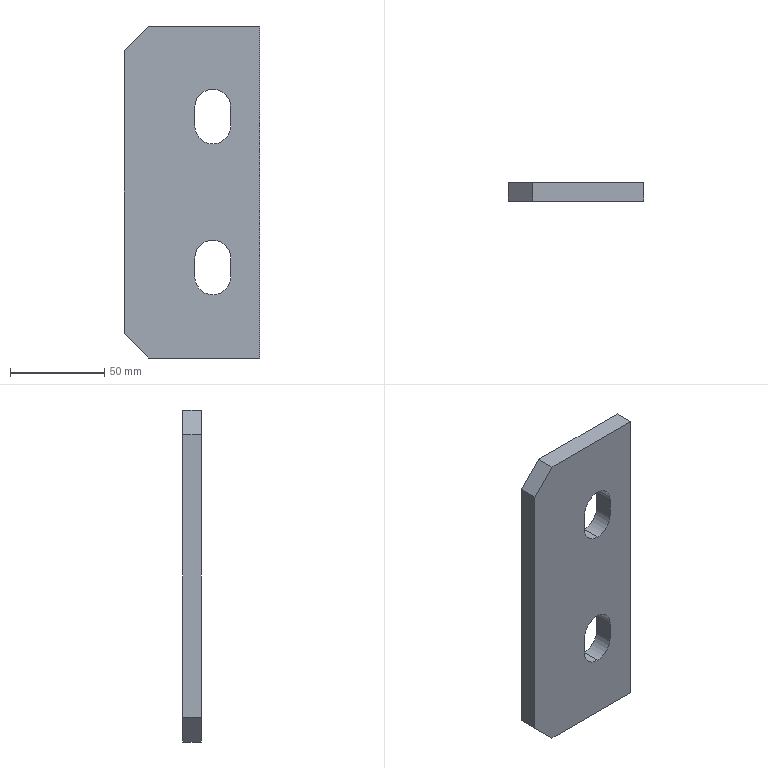Part | STEP file | 立柱填充筋Plate-194×150-1 | 1 solid | 18 faces | box 72 x 10 x 176 mm | volume 115559 mm3 | plane 12 | cylinder 6 | commonest cylinder face diameters 19 x6
STEP:
#1=CARTESIAN_POINT('',(0.,0.,0.));
#2=DIRECTION('',(0.,0.,1.));
#3=DIRECTION('',(1.,0.,0.));
#4=AXIS2_PLACEMENT_3D('',#1,#2,#3);
#5=CARTESIAN_POINT('',(56.5,0.,35.));
#6=VERTEX_POINT('',#5);
#7=CARTESIAN_POINT('',(56.5,10.,35.));
#8=VERTEX_POINT('',#7);
#9=CARTESIAN_POINT('',(56.5,40.,35.));
#10=DIRECTION('',(0.,1.,0.));
#11=VECTOR('',#10,1.);
#12=LINE('',#9,#11);
#13=CARTESIAN_POINT('',(47.,0.,35.));
#14=DIRECTION('',(0.,-1.,0.));
#15=DIRECTION('',(0.,0.,-1.));
#16=AXIS2_PLACEMENT_3D('',#13,#14,#15);
#17=CYLINDRICAL_SURFACE('',#16,9.5);
#18=CARTESIAN_POINT('',(1.571,-40.));
#19=DIRECTION('',(0.,-1.));
#20=VECTOR('',#19,1.);
#21=LINE('',#18,#20);
#22=(GEOMETRIC_REPRESENTATION_CONTEXT(2)PARAMETRIC_REPRESENTATION_CONTEXT()REPRESENTATION_CONTEXT('',''));
#23=DEFINITIONAL_REPRESENTATION('',(#21),#22);
#24=PCURVE('',#17,#23);
#25=CARTESIAN_POINT('',(56.5,40.,45.));
#26=DIRECTION('',(-1.,0.,0.));
#27=DIRECTION('',(0.,-1.,0.));
#28=AXIS2_PLACEMENT_3D('',#25,#26,#27);
#29=PLANE('',#28);
#30=CARTESIAN_POINT('',(0.,-10.));
#31=DIRECTION('',(-1.,0.));
#32=VECTOR('',#31,1.);
#33=LINE('',#30,#32);
#34=(GEOMETRIC_REPRESENTATION_CONTEXT(2)PARAMETRIC_REPRESENTATION_CONTEXT()REPRESENTATION_CONTEXT('',''));
#35=DEFINITIONAL_REPRESENTATION('',(#33),#34);
#36=PCURVE('',#29,#35);
#37=SURFACE_CURVE('',#12,(#24,#36),.PCURVE_S1.);
#38=EDGE_CURVE('',#6,#8,#37,.T.);
#39=ORIENTED_EDGE('',*,*,#38,.F.);
#40=CARTESIAN_POINT('',(47.,0.,25.5));
#41=VERTEX_POINT('',#40);
#42=CARTESIAN_POINT('',(47.,0.,35.));
#43=DIRECTION('',(0.,-1.,0.));
#44=DIRECTION('',(0.,0.,-1.));
#45=AXIS2_PLACEMENT_3D('',#42,#43,#44);
#46=CIRCLE('',#45,9.5);
#47=CARTESIAN_POINT('',(0.,0.));
#48=DIRECTION('',(1.,0.));
#49=VECTOR('',#48,1.);
#50=LINE('',#47,#49);
#51=(GEOMETRIC_REPRESENTATION_CONTEXT(2)PARAMETRIC_REPRESENTATION_CONTEXT()REPRESENTATION_CONTEXT('',''));
#52=DEFINITIONAL_REPRESENTATION('',(#50),#51);
#53=PCURVE('',#17,#52);
#54=CARTESIAN_POINT('',(0.,0.,0.));
#55=DIRECTION('',(0.,-1.,0.));
#56=DIRECTION('',(0.,0.,-1.));
#57=AXIS2_PLACEMENT_3D('',#54,#55,#56);
#58=PLANE('',#57);
#59=CARTESIAN_POINT('',(-35.,47.));
#60=DIRECTION('',(1.,0.));
#61=AXIS2_PLACEMENT_2D('',#59,#60);
#62=CIRCLE('',#61,9.5);
#63=(GEOMETRIC_REPRESENTATION_CONTEXT(2)PARAMETRIC_REPRESENTATION_CONTEXT()REPRESENTATION_CONTEXT('',''));
#64=DEFINITIONAL_REPRESENTATION('',(#62),#63);
#65=PCURVE('',#58,#64);
#66=SURFACE_CURVE('',#46,(#53,#65),.PCURVE_S1.);
#67=EDGE_CURVE('',#41,#6,#66,.T.);
#68=ORIENTED_EDGE('',*,*,#67,.F.);
#69=CARTESIAN_POINT('',(47.,10.,25.5));
#70=VERTEX_POINT('',#69);
#71=CARTESIAN_POINT('',(47.,0.,25.5));
#72=DIRECTION('',(0.,-1.,0.));
#73=VECTOR('',#72,1.);
#74=LINE('',#71,#73);
#75=CARTESIAN_POINT('',(0.,0.));
#76=DIRECTION('',(0.,1.));
#77=VECTOR('',#76,1.);
#78=LINE('',#75,#77);
#79=(GEOMETRIC_REPRESENTATION_CONTEXT(2)PARAMETRIC_REPRESENTATION_CONTEXT()REPRESENTATION_CONTEXT('',''));
#80=DEFINITIONAL_REPRESENTATION('',(#78),#79);
#81=PCURVE('',#17,#80);
#82=CARTESIAN_POINT('',(47.,0.,35.));
#83=DIRECTION('',(0.,-1.,0.));
#84=DIRECTION('',(0.,0.,-1.));
#85=AXIS2_PLACEMENT_3D('',#82,#83,#84);
#86=CYLINDRICAL_SURFACE('',#85,9.5);
#87=CARTESIAN_POINT('',(6.283,0.));
#88=DIRECTION('',(0.,1.));
#89=VECTOR('',#88,1.);
#90=LINE('',#87,#89);
#91=(GEOMETRIC_REPRESENTATION_CONTEXT(2)PARAMETRIC_REPRESENTATION_CONTEXT()REPRESENTATION_CONTEXT('',''));
#92=DEFINITIONAL_REPRESENTATION('',(#90),#91);
#93=PCURVE('',#86,#92);
#94=SURFACE_CURVE('',#74,(#81,#93),.PCURVE_S1.);
#95=EDGE_CURVE('',#70,#41,#94,.T.);
#96=ORIENTED_EDGE('',*,*,#95,.F.);
#97=CARTESIAN_POINT('',(47.,10.,35.));
#98=DIRECTION('',(0.,-1.,0.));
#99=DIRECTION('',(0.,0.,-1.));
#100=AXIS2_PLACEMENT_3D('',#97,#98,#99);
#101=CIRCLE('',#100,9.5);
#102=CARTESIAN_POINT('',(0.,-10.));
#103=DIRECTION('',(1.,0.));
#104=VECTOR('',#103,1.);
#105=LINE('',#102,#104);
#106=(GEOMETRIC_REPRESENTATION_CONTEXT(2)PARAMETRIC_REPRESENTATION_CONTEXT()REPRESENTATION_CONTEXT('',''));
#107=DEFINITIONAL_REPRESENTATION('',(#105),#106);
#108=PCURVE('',#17,#107);
#109=CARTESIAN_POINT('',(0.,10.,0.));
#110=DIRECTION('',(0.,-1.,0.));
#111=DIRECTION('',(0.,0.,-1.));
#112=AXIS2_PLACEMENT_3D('',#109,#110,#111);
#113=PLANE('',#112);
#114=CARTESIAN_POINT('',(-35.,47.));
#115=DIRECTION('',(1.,0.));
#116=AXIS2_PLACEMENT_2D('',#114,#115);
#117=CIRCLE('',#116,9.5);
#118=(GEOMETRIC_REPRESENTATION_CONTEXT(2)PARAMETRIC_REPRESENTATION_CONTEXT()REPRESENTATION_CONTEXT('',''));
#119=DEFINITIONAL_REPRESENTATION('',(#117),#118);
#120=PCURVE('',#113,#119);
#121=SURFACE_CURVE('',#101,(#108,#120),.PCURVE_S1.);
#122=EDGE_CURVE('',#70,#8,#121,.T.);
#123=ORIENTED_EDGE('',*,*,#122,.T.);
#124=EDGE_LOOP('',(#39,#68,#96,#123));
#125=FACE_BOUND('',#124,.F.);
#126=ADVANCED_FACE('',(#125),#17,.F.);
#127=CARTESIAN_POINT('',(56.5,0.,-45.));
#128=VERTEX_POINT('',#127);
#129=CARTESIAN_POINT('',(56.5,10.,-45.));
#130=VERTEX_POINT('',#129);
#131=CARTESIAN_POINT('',(56.5,40.,-45.));
#132=DIRECTION('',(0.,1.,0.));
#133=VECTOR('',#132,1.);
#134=LINE('',#131,#133);
#135=CARTESIAN_POINT('',(47.,0.,-45.));
#136=DIRECTION('',(0.,-1.,0.));
#137=DIRECTION('',(0.,0.,-1.));
#138=AXIS2_PLACEMENT_3D('',#135,#136,#137);
#139=CYLINDRICAL_SURFACE('',#138,9.5);
#140=CARTESIAN_POINT('',(1.571,-40.));
#141=DIRECTION('',(0.,-1.));
#142=VECTOR('',#141,1.);
#143=LINE('',#140,#142);
#144=(GEOMETRIC_REPRESENTATION_CONTEXT(2)PARAMETRIC_REPRESENTATION_CONTEXT()REPRESENTATION_CONTEXT('',''));
#145=DEFINITIONAL_REPRESENTATION('',(#143),#144);
#146=PCURVE('',#139,#145);
#147=CARTESIAN_POINT('',(56.5,40.,-35.));
#148=DIRECTION('',(-1.,0.,0.));
#149=DIRECTION('',(0.,-1.,0.));
#150=AXIS2_PLACEMENT_3D('',#147,#148,#149);
#151=PLANE('',#150);
#152=CARTESIAN_POINT('',(0.,-10.));
#153=DIRECTION('',(-1.,0.));
#154=VECTOR('',#153,1.);
#155=LINE('',#152,#154);
#156=(GEOMETRIC_REPRESENTATION_CONTEXT(2)PARAMETRIC_REPRESENTATION_CONTEXT()REPRESENTATION_CONTEXT('',''));
#157=DEFINITIONAL_REPRESENTATION('',(#155),#156);
#158=PCURVE('',#151,#157);
#159=SURFACE_CURVE('',#134,(#146,#158),.PCURVE_S1.);
#160=EDGE_CURVE('',#128,#130,#159,.T.);
#161=ORIENTED_EDGE('',*,*,#160,.F.);
#162=CARTESIAN_POINT('',(47.,0.,-54.5));
#163=VERTEX_POINT('',#162);
#164=CARTESIAN_POINT('',(47.,0.,-45.));
#165=DIRECTION('',(0.,-1.,0.));
#166=DIRECTION('',(0.,0.,-1.));
#167=AXIS2_PLACEMENT_3D('',#164,#165,#166);
#168=CIRCLE('',#167,9.5);
#169=CARTESIAN_POINT('',(0.,0.));
#170=DIRECTION('',(1.,0.));
#171=VECTOR('',#170,1.);
#172=LINE('',#169,#171);
#173=(GEOMETRIC_REPRESENTATION_CONTEXT(2)PARAMETRIC_REPRESENTATION_CONTEXT()REPRESENTATION_CONTEXT('',''));
#174=DEFINITIONAL_REPRESENTATION('',(#172),#173);
#175=PCURVE('',#139,#174);
#176=CARTESIAN_POINT('',(45.,47.));
#177=DIRECTION('',(1.,0.));
#178=AXIS2_PLACEMENT_2D('',#176,#177);
#179=CIRCLE('',#178,9.5);
#180=(GEOMETRIC_REPRESENTATION_CONTEXT(2)PARAMETRIC_REPRESENTATION_CONTEXT()REPRESENTATION_CONTEXT('',''));
#181=DEFINITIONAL_REPRESENTATION('',(#179),#180);
#182=PCURVE('',#58,#181);
#183=SURFACE_CURVE('',#168,(#175,#182),.PCURVE_S1.);
#184=EDGE_CURVE('',#163,#128,#183,.T.);
#185=ORIENTED_EDGE('',*,*,#184,.F.);
#186=CARTESIAN_POINT('',(47.,10.,-54.5));
#187=VERTEX_POINT('',#186);
#188=CARTESIAN_POINT('',(47.,0.,-54.5));
#189=DIRECTION('',(0.,-1.,0.));
#190=VECTOR('',#189,1.);
#191=LINE('',#188,#190);
#192=CARTESIAN_POINT('',(0.,0.));
#193=DIRECTION('',(0.,1.));
#194=VECTOR('',#193,1.);
#195=LINE('',#192,#194);
#196=(GEOMETRIC_REPRESENTATION_CONTEXT(2)PARAMETRIC_REPRESENTATION_CONTEXT()REPRESENTATION_CONTEXT('',''));
#197=DEFINITIONAL_REPRESENTATION('',(#195),#196);
#198=PCURVE('',#139,#197);
#199=CARTESIAN_POINT('',(47.,0.,-45.));
#200=DIRECTION('',(0.,-1.,0.));
#201=DIRECTION('',(0.,0.,-1.));
#202=AXIS2_PLACEMENT_3D('',#199,#200,#201);
#203=CYLINDRICAL_SURFACE('',#202,9.5);
#204=CARTESIAN_POINT('',(6.283,0.));
#205=DIRECTION('',(0.,1.));
#206=VECTOR('',#205,1.);
#207=LINE('',#204,#206);
#208=(GEOMETRIC_REPRESENTATION_CONTEXT(2)PARAMETRIC_REPRESENTATION_CONTEXT()REPRESENTATION_CONTEXT('',''));
#209=DEFINITIONAL_REPRESENTATION('',(#207),#208);
#210=PCURVE('',#203,#209);
#211=SURFACE_CURVE('',#191,(#198,#210),.PCURVE_S1.);
#212=EDGE_CURVE('',#187,#163,#211,.T.);
#213=ORIENTED_EDGE('',*,*,#212,.F.);
#214=CARTESIAN_POINT('',(47.,10.,-45.));
#215=DIRECTION('',(0.,-1.,0.));
#216=DIRECTION('',(0.,0.,-1.));
#217=AXIS2_PLACEMENT_3D('',#214,#215,#216);
#218=CIRCLE('',#217,9.5);
#219=CARTESIAN_POINT('',(0.,-10.));
#220=DIRECTION('',(1.,0.));
#221=VECTOR('',#220,1.);
#222=LINE('',#219,#221);
#223=(GEOMETRIC_REPRESENTATION_CONTEXT(2)PARAMETRIC_REPRESENTATION_CONTEXT()REPRESENTATION_CONTEXT('',''));
#224=DEFINITIONAL_REPRESENTATION('',(#222),#223);
#225=PCURVE('',#139,#224);
#226=CARTESIAN_POINT('',(45.,47.));
#227=DIRECTION('',(1.,0.));
#228=AXIS2_PLACEMENT_2D('',#226,#227);
#229=CIRCLE('',#228,9.5);
#230=(GEOMETRIC_REPRESENTATION_CONTEXT(2)PARAMETRIC_REPRESENTATION_CONTEXT()REPRESENTATION_CONTEXT('',''));
#231=DEFINITIONAL_REPRESENTATION('',(#229),#230);
#232=PCURVE('',#113,#231);
#233=SURFACE_CURVE('',#218,(#225,#232),.PCURVE_S1.);
#234=EDGE_CURVE('',#187,#130,#233,.T.);
#235=ORIENTED_EDGE('',*,*,#234,.T.);
#236=EDGE_LOOP('',(#161,#185,#213,#235));
#237=FACE_BOUND('',#236,.F.);
#238=ADVANCED_FACE('',(#237),#139,.F.);
#239=CARTESIAN_POINT('',(13.,0.,88.));
#240=VERTEX_POINT('',#239);
#241=CARTESIAN_POINT('',(72.,0.,88.));
#242=VERTEX_POINT('',#241);
#243=CARTESIAN_POINT('',(72.,0.,88.));
#244=DIRECTION('',(1.,0.,0.));
#245=VECTOR('',#244,1.);
#246=LINE('',#243,#245);
#247=CARTESIAN_POINT('',(-88.,72.));
#248=DIRECTION('',(0.,1.));
#249=VECTOR('',#248,1.);
#250=LINE('',#247,#249);
#251=(GEOMETRIC_REPRESENTATION_CONTEXT(2)PARAMETRIC_REPRESENTATION_CONTEXT()REPRESENTATION_CONTEXT('',''));
#252=DEFINITIONAL_REPRESENTATION('',(#250),#251);
#253=PCURVE('',#58,#252);
#254=CARTESIAN_POINT('',(72.,10.,88.));
#255=DIRECTION('',(0.,0.,-1.));
#256=DIRECTION('',(-1.,0.,0.));
#257=AXIS2_PLACEMENT_3D('',#254,#255,#256);
#258=PLANE('',#257);
#259=CARTESIAN_POINT('',(0.,-10.));
#260=DIRECTION('',(-1.,0.));
#261=VECTOR('',#260,1.);
#262=LINE('',#259,#261);
#263=(GEOMETRIC_REPRESENTATION_CONTEXT(2)PARAMETRIC_REPRESENTATION_CONTEXT()REPRESENTATION_CONTEXT('',''));
#264=DEFINITIONAL_REPRESENTATION('',(#262),#263);
#265=PCURVE('',#258,#264);
#266=SURFACE_CURVE('',#246,(#253,#265),.PCURVE_S1.);
#267=EDGE_CURVE('',#240,#242,#266,.T.);
#268=ORIENTED_EDGE('',*,*,#267,.F.);
#269=CARTESIAN_POINT('',(0.,0.,75.));
#270=VERTEX_POINT('',#269);
#271=CARTESIAN_POINT('',(-37.5,0.,37.5));
#272=DIRECTION('',(-0.7071,0.,-0.7071));
#273=VECTOR('',#272,1.);
#274=LINE('',#271,#273);
#275=CARTESIAN_POINT('',(-37.5,-37.5));
#276=DIRECTION('',(0.7071,-0.7071));
#277=VECTOR('',#276,1.);
#278=LINE('',#275,#277);
#279=(GEOMETRIC_REPRESENTATION_CONTEXT(2)PARAMETRIC_REPRESENTATION_CONTEXT()REPRESENTATION_CONTEXT('',''));
#280=DEFINITIONAL_REPRESENTATION('',(#278),#279);
#281=PCURVE('',#58,#280);
#282=CARTESIAN_POINT('',(13.,10.,88.));
#283=DIRECTION('',(0.7071,0.,-0.7071));
#284=DIRECTION('',(0.,-1.,0.));
#285=AXIS2_PLACEMENT_3D('',#282,#283,#284);
#286=PLANE('',#285);
#287=CARTESIAN_POINT('',(10.,71.418));
#288=DIRECTION('',(0.,1.));
#289=VECTOR('',#288,1.);
#290=LINE('',#287,#289);
#291=(GEOMETRIC_REPRESENTATION_CONTEXT(2)PARAMETRIC_REPRESENTATION_CONTEXT()REPRESENTATION_CONTEXT('',''));
#292=DEFINITIONAL_REPRESENTATION('',(#290),#291);
#293=PCURVE('',#286,#292);
#294=SURFACE_CURVE('',#274,(#281,#293),.PCURVE_S1.);
#295=EDGE_CURVE('',#240,#270,#294,.T.);
#296=ORIENTED_EDGE('',*,*,#295,.T.);
#297=CARTESIAN_POINT('',(0.,0.,-75.));
#298=VERTEX_POINT('',#297);
#299=CARTESIAN_POINT('',(0.,0.,88.));
#300=DIRECTION('',(0.,0.,1.));
#301=VECTOR('',#300,1.);
#302=LINE('',#299,#301);
#303=CARTESIAN_POINT('',(-88.,0.));
#304=DIRECTION('',(-1.,0.));
#305=VECTOR('',#304,1.);
#306=LINE('',#303,#305);
#307=(GEOMETRIC_REPRESENTATION_CONTEXT(2)PARAMETRIC_REPRESENTATION_CONTEXT()REPRESENTATION_CONTEXT('',''));
#308=DEFINITIONAL_REPRESENTATION('',(#306),#307);
#309=PCURVE('',#58,#308);
#310=CARTESIAN_POINT('',(0.,10.,88.));
#311=DIRECTION('',(1.,0.,0.));
#312=DIRECTION('',(0.,0.,-1.));
#313=AXIS2_PLACEMENT_3D('',#310,#311,#312);
#314=PLANE('',#313);
#315=CARTESIAN_POINT('',(0.,-10.));
#316=DIRECTION('',(-1.,0.));
#317=VECTOR('',#316,1.);
#318=LINE('',#315,#317);
#319=(GEOMETRIC_REPRESENTATION_CONTEXT(2)PARAMETRIC_REPRESENTATION_CONTEXT()REPRESENTATION_CONTEXT('',''));
#320=DEFINITIONAL_REPRESENTATION('',(#318),#319);
#321=PCURVE('',#314,#320);
#322=SURFACE_CURVE('',#302,(#309,#321),.PCURVE_S1.);
#323=EDGE_CURVE('',#298,#270,#322,.T.);
#324=ORIENTED_EDGE('',*,*,#323,.F.);
#325=CARTESIAN_POINT('',(13.,0.,-88.));
#326=VERTEX_POINT('',#325);
#327=CARTESIAN_POINT('',(-37.5,0.,-37.5));
#328=DIRECTION('',(0.7071,0.,-0.7071));
#329=VECTOR('',#328,1.);
#330=LINE('',#327,#329);
#331=CARTESIAN_POINT('',(37.5,-37.5));
#332=DIRECTION('',(0.7071,0.7071));
#333=VECTOR('',#332,1.);
#334=LINE('',#331,#333);
#335=(GEOMETRIC_REPRESENTATION_CONTEXT(2)PARAMETRIC_REPRESENTATION_CONTEXT()REPRESENTATION_CONTEXT('',''));
#336=DEFINITIONAL_REPRESENTATION('',(#334),#335);
#337=PCURVE('',#58,#336);
#338=CARTESIAN_POINT('',(0.,10.,-75.));
#339=DIRECTION('',(0.7071,0.,0.7071));
#340=DIRECTION('',(0.,-1.,0.));
#341=AXIS2_PLACEMENT_3D('',#338,#339,#340);
#342=PLANE('',#341);
#343=CARTESIAN_POINT('',(10.,-53.033));
#344=DIRECTION('',(0.,1.));
#345=VECTOR('',#344,1.);
#346=LINE('',#343,#345);
#347=(GEOMETRIC_REPRESENTATION_CONTEXT(2)PARAMETRIC_REPRESENTATION_CONTEXT()REPRESENTATION_CONTEXT('',''));
#348=DEFINITIONAL_REPRESENTATION('',(#346),#347);
#349=PCURVE('',#342,#348);
#350=SURFACE_CURVE('',#330,(#337,#349),.PCURVE_S1.);
#351=EDGE_CURVE('',#298,#326,#350,.T.);
#352=ORIENTED_EDGE('',*,*,#351,.T.);
#353=CARTESIAN_POINT('',(72.,0.,-88.));
#354=VERTEX_POINT('',#353);
#355=CARTESIAN_POINT('',(0.,0.,-88.));
#356=DIRECTION('',(-1.,0.,0.));
#357=VECTOR('',#356,1.);
#358=LINE('',#355,#357);
#359=CARTESIAN_POINT('',(88.,0.));
#360=DIRECTION('',(0.,-1.));
#361=VECTOR('',#360,1.);
#362=LINE('',#359,#361);
#363=(GEOMETRIC_REPRESENTATION_CONTEXT(2)PARAMETRIC_REPRESENTATION_CONTEXT()REPRESENTATION_CONTEXT('',''));
#364=DEFINITIONAL_REPRESENTATION('',(#362),#363);
#365=PCURVE('',#58,#364);
#366=CARTESIAN_POINT('',(0.,10.,-88.));
#367=DIRECTION('',(0.,0.,1.));
#368=DIRECTION('',(1.,0.,0.));
#369=AXIS2_PLACEMENT_3D('',#366,#367,#368);
#370=PLANE('',#369);
#371=CARTESIAN_POINT('',(0.,-10.));
#372=DIRECTION('',(-1.,0.));
#373=VECTOR('',#372,1.);
#374=LINE('',#371,#373);
#375=(GEOMETRIC_REPRESENTATION_CONTEXT(2)PARAMETRIC_REPRESENTATION_CONTEXT()REPRESENTATION_CONTEXT('',''));
#376=DEFINITIONAL_REPRESENTATION('',(#374),#375);
#377=PCURVE('',#370,#376);
#378=SURFACE_CURVE('',#358,(#365,#377),.PCURVE_S1.);
#379=EDGE_CURVE('',#354,#326,#378,.T.);
#380=ORIENTED_EDGE('',*,*,#379,.F.);
#381=CARTESIAN_POINT('',(72.,0.,-88.));
#382=DIRECTION('',(0.,0.,-1.));
#383=VECTOR('',#382,1.);
#384=LINE('',#381,#383);
#385=CARTESIAN_POINT('',(88.,72.));
#386=DIRECTION('',(1.,0.));
#387=VECTOR('',#386,1.);
#388=LINE('',#385,#387);
#389=(GEOMETRIC_REPRESENTATION_CONTEXT(2)PARAMETRIC_REPRESENTATION_CONTEXT()REPRESENTATION_CONTEXT('',''));
#390=DEFINITIONAL_REPRESENTATION('',(#388),#389);
#391=PCURVE('',#58,#390);
#392=CARTESIAN_POINT('',(72.,10.,-88.));
#393=DIRECTION('',(-1.,0.,0.));
#394=DIRECTION('',(0.,0.,1.));
#395=AXIS2_PLACEMENT_3D('',#392,#393,#394);
#396=PLANE('',#395);
#397=CARTESIAN_POINT('',(0.,-10.));
#398=DIRECTION('',(-1.,0.));
#399=VECTOR('',#398,1.);
#400=LINE('',#397,#399);
#401=(GEOMETRIC_REPRESENTATION_CONTEXT(2)PARAMETRIC_REPRESENTATION_CONTEXT()REPRESENTATION_CONTEXT('',''));
#402=DEFINITIONAL_REPRESENTATION('',(#400),#401);
#403=PCURVE('',#396,#402);
#404=SURFACE_CURVE('',#384,(#391,#403),.PCURVE_S1.);
#405=EDGE_CURVE('',#242,#354,#404,.T.);
#406=ORIENTED_EDGE('',*,*,#405,.F.);
#407=EDGE_LOOP('',(#268,#296,#324,#352,#380,#406));
#408=FACE_BOUND('',#407,.T.);
#409=CARTESIAN_POINT('',(56.5,0.,-35.));
#410=VERTEX_POINT('',#409);
#411=CARTESIAN_POINT('',(37.5,0.,-35.));
#412=VERTEX_POINT('',#411);
#413=CARTESIAN_POINT('',(47.,0.,-35.));
#414=DIRECTION('',(0.,-1.,0.));
#415=DIRECTION('',(0.,0.,-1.));
#416=AXIS2_PLACEMENT_3D('',#413,#414,#415);
#417=CIRCLE('',#416,9.5);
#418=CARTESIAN_POINT('',(35.,47.));
#419=DIRECTION('',(1.,0.));
#420=AXIS2_PLACEMENT_2D('',#418,#419);
#421=CIRCLE('',#420,9.5);
#422=(GEOMETRIC_REPRESENTATION_CONTEXT(2)PARAMETRIC_REPRESENTATION_CONTEXT()REPRESENTATION_CONTEXT('',''));
#423=DEFINITIONAL_REPRESENTATION('',(#421),#422);
#424=PCURVE('',#58,#423);
#425=CARTESIAN_POINT('',(47.,0.,-35.));
#426=DIRECTION('',(0.,-1.,0.));
#427=DIRECTION('',(0.,0.,-1.));
#428=AXIS2_PLACEMENT_3D('',#425,#426,#427);
#429=CYLINDRICAL_SURFACE('',#428,9.5);
#430=CARTESIAN_POINT('',(0.,0.));
#431=DIRECTION('',(1.,0.));
#432=VECTOR('',#431,1.);
#433=LINE('',#430,#432);
#434=(GEOMETRIC_REPRESENTATION_CONTEXT(2)PARAMETRIC_REPRESENTATION_CONTEXT()REPRESENTATION_CONTEXT('',''));
#435=DEFINITIONAL_REPRESENTATION('',(#433),#434);
#436=PCURVE('',#429,#435);
#437=SURFACE_CURVE('',#417,(#424,#436),.PCURVE_S1.);
#438=EDGE_CURVE('',#410,#412,#437,.T.);
#439=ORIENTED_EDGE('',*,*,#438,.F.);
#440=CARTESIAN_POINT('',(56.5,0.,-35.));
#441=DIRECTION('',(0.,0.,-1.));
#442=VECTOR('',#441,1.);
#443=LINE('',#440,#442);
#444=CARTESIAN_POINT('',(35.,56.5));
#445=DIRECTION('',(1.,0.));
#446=VECTOR('',#445,1.);
#447=LINE('',#444,#446);
#448=(GEOMETRIC_REPRESENTATION_CONTEXT(2)PARAMETRIC_REPRESENTATION_CONTEXT()REPRESENTATION_CONTEXT('',''));
#449=DEFINITIONAL_REPRESENTATION('',(#447),#448);
#450=PCURVE('',#58,#449);
#451=CARTESIAN_POINT('',(40.,0.));
#452=DIRECTION('',(0.,-1.));
#453=VECTOR('',#452,1.);
#454=LINE('',#451,#453);
#455=(GEOMETRIC_REPRESENTATION_CONTEXT(2)PARAMETRIC_REPRESENTATION_CONTEXT()REPRESENTATION_CONTEXT('',''));
#456=DEFINITIONAL_REPRESENTATION('',(#454),#455);
#457=PCURVE('',#151,#456);
#458=SURFACE_CURVE('',#443,(#450,#457),.PCURVE_S1.);
#459=EDGE_CURVE('',#410,#128,#458,.T.);
#460=ORIENTED_EDGE('',*,*,#459,.T.);
#461=ORIENTED_EDGE('',*,*,#184,.F.);
#462=CARTESIAN_POINT('',(37.5,0.,-45.));
#463=VERTEX_POINT('',#462);
#464=CARTESIAN_POINT('',(47.,0.,-45.));
#465=DIRECTION('',(0.,-1.,0.));
#466=DIRECTION('',(0.,0.,-1.));
#467=AXIS2_PLACEMENT_3D('',#464,#465,#466);
#468=CIRCLE('',#467,9.5);
#469=CARTESIAN_POINT('',(45.,47.));
#470=DIRECTION('',(1.,0.));
#471=AXIS2_PLACEMENT_2D('',#469,#470);
#472=CIRCLE('',#471,9.5);
#473=(GEOMETRIC_REPRESENTATION_CONTEXT(2)PARAMETRIC_REPRESENTATION_CONTEXT()REPRESENTATION_CONTEXT('',''));
#474=DEFINITIONAL_REPRESENTATION('',(#472),#473);
#475=PCURVE('',#58,#474);
#476=CARTESIAN_POINT('',(0.,0.));
#477=DIRECTION('',(1.,0.));
#478=VECTOR('',#477,1.);
#479=LINE('',#476,#478);
#480=(GEOMETRIC_REPRESENTATION_CONTEXT(2)PARAMETRIC_REPRESENTATION_CONTEXT()REPRESENTATION_CONTEXT('',''));
#481=DEFINITIONAL_REPRESENTATION('',(#479),#480);
#482=PCURVE('',#203,#481);
#483=SURFACE_CURVE('',#468,(#475,#482),.PCURVE_S1.);
#484=EDGE_CURVE('',#463,#163,#483,.T.);
#485=ORIENTED_EDGE('',*,*,#484,.F.);
#486=CARTESIAN_POINT('',(37.5,0.,-35.));
#487=DIRECTION('',(0.,0.,-1.));
#488=VECTOR('',#487,1.);
#489=LINE('',#486,#488);
#490=CARTESIAN_POINT('',(35.,37.5));
#491=DIRECTION('',(1.,0.));
#492=VECTOR('',#491,1.);
#493=LINE('',#490,#492);
#494=(GEOMETRIC_REPRESENTATION_CONTEXT(2)PARAMETRIC_REPRESENTATION_CONTEXT()REPRESENTATION_CONTEXT('',''));
#495=DEFINITIONAL_REPRESENTATION('',(#493),#494);
#496=PCURVE('',#58,#495);
#497=CARTESIAN_POINT('',(37.5,0.,-35.));
#498=DIRECTION('',(-1.,0.,0.));
#499=DIRECTION('',(0.,0.,1.));
#500=AXIS2_PLACEMENT_3D('',#497,#498,#499);
#501=PLANE('',#500);
#502=CARTESIAN_POINT('',(0.,0.));
#503=DIRECTION('',(-1.,0.));
#504=VECTOR('',#503,1.);
#505=LINE('',#502,#504);
#506=(GEOMETRIC_REPRESENTATION_CONTEXT(2)PARAMETRIC_REPRESENTATION_CONTEXT()REPRESENTATION_CONTEXT('',''));
#507=DEFINITIONAL_REPRESENTATION('',(#505),#506);
#508=PCURVE('',#501,#507);
#509=SURFACE_CURVE('',#489,(#496,#508),.PCURVE_S1.);
#510=EDGE_CURVE('',#412,#463,#509,.T.);
#511=ORIENTED_EDGE('',*,*,#510,.F.);
#512=EDGE_LOOP('',(#439,#460,#461,#485,#511));
#513=FACE_BOUND('',#512,.T.);
#514=CARTESIAN_POINT('',(56.5,0.,45.));
#515=VERTEX_POINT('',#514);
#516=CARTESIAN_POINT('',(37.5,0.,45.));
#517=VERTEX_POINT('',#516);
#518=CARTESIAN_POINT('',(47.,0.,45.));
#519=DIRECTION('',(0.,-1.,0.));
#520=DIRECTION('',(0.,0.,-1.));
#521=AXIS2_PLACEMENT_3D('',#518,#519,#520);
#522=CIRCLE('',#521,9.5);
#523=CARTESIAN_POINT('',(-45.,47.));
#524=DIRECTION('',(1.,0.));
#525=AXIS2_PLACEMENT_2D('',#523,#524);
#526=CIRCLE('',#525,9.5);
#527=(GEOMETRIC_REPRESENTATION_CONTEXT(2)PARAMETRIC_REPRESENTATION_CONTEXT()REPRESENTATION_CONTEXT('',''));
#528=DEFINITIONAL_REPRESENTATION('',(#526),#527);
#529=PCURVE('',#58,#528);
#530=CARTESIAN_POINT('',(47.,0.,45.));
#531=DIRECTION('',(0.,-1.,0.));
#532=DIRECTION('',(0.,0.,-1.));
#533=AXIS2_PLACEMENT_3D('',#530,#531,#532);
#534=CYLINDRICAL_SURFACE('',#533,9.5);
#535=CARTESIAN_POINT('',(0.,0.));
#536=DIRECTION('',(1.,0.));
#537=VECTOR('',#536,1.);
#538=LINE('',#535,#537);
#539=(GEOMETRIC_REPRESENTATION_CONTEXT(2)PARAMETRIC_REPRESENTATION_CONTEXT()REPRESENTATION_CONTEXT('',''));
#540=DEFINITIONAL_REPRESENTATION('',(#538),#539);
#541=PCURVE('',#534,#540);
#542=SURFACE_CURVE('',#522,(#529,#541),.PCURVE_S1.);
#543=EDGE_CURVE('',#515,#517,#542,.T.);
#544=ORIENTED_EDGE('',*,*,#543,.F.);
#545=CARTESIAN_POINT('',(56.5,0.,45.));
#546=DIRECTION('',(0.,0.,-1.));
#547=VECTOR('',#546,1.);
#548=LINE('',#545,#547);
#549=CARTESIAN_POINT('',(-45.,56.5));
#550=DIRECTION('',(1.,0.));
#551=VECTOR('',#550,1.);
#552=LINE('',#549,#551);
#553=(GEOMETRIC_REPRESENTATION_CONTEXT(2)PARAMETRIC_REPRESENTATION_CONTEXT()REPRESENTATION_CONTEXT('',''));
#554=DEFINITIONAL_REPRESENTATION('',(#552),#553);
#555=PCURVE('',#58,#554);
#556=CARTESIAN_POINT('',(40.,0.));
#557=DIRECTION('',(0.,-1.));
#558=VECTOR('',#557,1.);
#559=LINE('',#556,#558);
#560=(GEOMETRIC_REPRESENTATION_CONTEXT(2)PARAMETRIC_REPRESENTATION_CONTEXT()REPRESENTATION_CONTEXT('',''));
#561=DEFINITIONAL_REPRESENTATION('',(#559),#560);
#562=PCURVE('',#29,#561);
#563=SURFACE_CURVE('',#548,(#555,#562),.PCURVE_S1.);
#564=EDGE_CURVE('',#515,#6,#563,.T.);
#565=ORIENTED_EDGE('',*,*,#564,.T.);
#566=ORIENTED_EDGE('',*,*,#67,.F.);
#567=CARTESIAN_POINT('',(37.5,0.,35.));
#568=VERTEX_POINT('',#567);
#569=CARTESIAN_POINT('',(47.,0.,35.));
#570=DIRECTION('',(0.,-1.,0.));
#571=DIRECTION('',(0.,0.,-1.));
#572=AXIS2_PLACEMENT_3D('',#569,#570,#571);
#573=CIRCLE('',#572,9.5);
#574=CARTESIAN_POINT('',(-35.,47.));
#575=DIRECTION('',(1.,0.));
#576=AXIS2_PLACEMENT_2D('',#574,#575);
#577=CIRCLE('',#576,9.5);
#578=(GEOMETRIC_REPRESENTATION_CONTEXT(2)PARAMETRIC_REPRESENTATION_CONTEXT()REPRESENTATION_CONTEXT('',''));
#579=DEFINITIONAL_REPRESENTATION('',(#577),#578);
#580=PCURVE('',#58,#579);
#581=CARTESIAN_POINT('',(0.,0.));
#582=DIRECTION('',(1.,0.));
#583=VECTOR('',#582,1.);
#584=LINE('',#581,#583);
#585=(GEOMETRIC_REPRESENTATION_CONTEXT(2)PARAMETRIC_REPRESENTATION_CONTEXT()REPRESENTATION_CONTEXT('',''));
#586=DEFINITIONAL_REPRESENTATION('',(#584),#585);
#587=PCURVE('',#86,#586);
#588=SURFACE_CURVE('',#573,(#580,#587),.PCURVE_S1.);
#589=EDGE_CURVE('',#568,#41,#588,.T.);
#590=ORIENTED_EDGE('',*,*,#589,.F.);
#591=CARTESIAN_POINT('',(37.5,0.,45.));
#592=DIRECTION('',(0.,0.,-1.));
#593=VECTOR('',#592,1.);
#594=LINE('',#591,#593);
#595=CARTESIAN_POINT('',(-45.,37.5));
#596=DIRECTION('',(1.,0.));
#597=VECTOR('',#596,1.);
#598=LINE('',#595,#597);
#599=(GEOMETRIC_REPRESENTATION_CONTEXT(2)PARAMETRIC_REPRESENTATION_CONTEXT()REPRESENTATION_CONTEXT('',''));
#600=DEFINITIONAL_REPRESENTATION('',(#598),#599);
#601=PCURVE('',#58,#600);
#602=CARTESIAN_POINT('',(37.5,0.,45.));
#603=DIRECTION('',(-1.,0.,0.));
#604=DIRECTION('',(0.,0.,1.));
#605=AXIS2_PLACEMENT_3D('',#602,#603,#604);
#606=PLANE('',#605);
#607=CARTESIAN_POINT('',(0.,0.));
#608=DIRECTION('',(-1.,0.));
#609=VECTOR('',#608,1.);
#610=LINE('',#607,#609);
#611=(GEOMETRIC_REPRESENTATION_CONTEXT(2)PARAMETRIC_REPRESENTATION_CONTEXT()REPRESENTATION_CONTEXT('',''));
#612=DEFINITIONAL_REPRESENTATION('',(#610),#611);
#613=PCURVE('',#606,#612);
#614=SURFACE_CURVE('',#594,(#601,#613),.PCURVE_S1.);
#615=EDGE_CURVE('',#517,#568,#614,.T.);
#616=ORIENTED_EDGE('',*,*,#615,.F.);
#617=EDGE_LOOP('',(#544,#565,#566,#590,#616));
#618=FACE_BOUND('',#617,.T.);
#619=ADVANCED_FACE('',(#408,#513,#618),#58,.T.);
#620=CARTESIAN_POINT('',(56.5,10.,45.));
#621=VERTEX_POINT('',#620);
#622=CARTESIAN_POINT('',(56.5,10.,0.));
#623=DIRECTION('',(0.,0.,-1.));
#624=VECTOR('',#623,1.);
#625=LINE('',#622,#624);
#626=CARTESIAN_POINT('',(0.,56.5));
#627=DIRECTION('',(1.,0.));
#628=VECTOR('',#627,1.);
#629=LINE('',#626,#628);
#630=(GEOMETRIC_REPRESENTATION_CONTEXT(2)PARAMETRIC_REPRESENTATION_CONTEXT()REPRESENTATION_CONTEXT('',''));
#631=DEFINITIONAL_REPRESENTATION('',(#629),#630);
#632=PCURVE('',#113,#631);
#633=CARTESIAN_POINT('',(30.,-45.));
#634=DIRECTION('',(0.,-1.));
#635=VECTOR('',#634,1.);
#636=LINE('',#633,#635);
#637=(GEOMETRIC_REPRESENTATION_CONTEXT(2)PARAMETRIC_REPRESENTATION_CONTEXT()REPRESENTATION_CONTEXT('',''));
#638=DEFINITIONAL_REPRESENTATION('',(#636),#637);
#639=PCURVE('',#29,#638);
#640=SURFACE_CURVE('',#625,(#632,#639),.PCURVE_S1.);
#641=EDGE_CURVE('',#621,#8,#640,.T.);
#642=ORIENTED_EDGE('',*,*,#641,.F.);
#643=CARTESIAN_POINT('',(37.5,10.,45.));
#644=VERTEX_POINT('',#643);
#645=CARTESIAN_POINT('',(47.,10.,45.));
#646=DIRECTION('',(0.,-1.,0.));
#647=DIRECTION('',(0.,0.,-1.));
#648=AXIS2_PLACEMENT_3D('',#645,#646,#647);
#649=CIRCLE('',#648,9.5);
#650=CARTESIAN_POINT('',(-45.,47.));
#651=DIRECTION('',(1.,0.));
#652=AXIS2_PLACEMENT_2D('',#650,#651);
#653=CIRCLE('',#652,9.5);
#654=(GEOMETRIC_REPRESENTATION_CONTEXT(2)PARAMETRIC_REPRESENTATION_CONTEXT()REPRESENTATION_CONTEXT('',''));
#655=DEFINITIONAL_REPRESENTATION('',(#653),#654);
#656=PCURVE('',#113,#655);
#657=CARTESIAN_POINT('',(0.,-10.));
#658=DIRECTION('',(1.,0.));
#659=VECTOR('',#658,1.);
#660=LINE('',#657,#659);
#661=(GEOMETRIC_REPRESENTATION_CONTEXT(2)PARAMETRIC_REPRESENTATION_CONTEXT()REPRESENTATION_CONTEXT('',''));
#662=DEFINITIONAL_REPRESENTATION('',(#660),#661);
#663=PCURVE('',#534,#662);
#664=SURFACE_CURVE('',#649,(#656,#663),.PCURVE_S1.);
#665=EDGE_CURVE('',#621,#644,#664,.T.);
#666=ORIENTED_EDGE('',*,*,#665,.T.);
#667=CARTESIAN_POINT('',(37.5,10.,35.));
#668=VERTEX_POINT('',#667);
#669=CARTESIAN_POINT('',(37.5,10.,0.));
#670=DIRECTION('',(0.,0.,-1.));
#671=VECTOR('',#670,1.);
#672=LINE('',#669,#671);
#673=CARTESIAN_POINT('',(0.,37.5));
#674=DIRECTION('',(1.,0.));
#675=VECTOR('',#674,1.);
#676=LINE('',#673,#675);
#677=(GEOMETRIC_REPRESENTATION_CONTEXT(2)PARAMETRIC_REPRESENTATION_CONTEXT()REPRESENTATION_CONTEXT('',''));
#678=DEFINITIONAL_REPRESENTATION('',(#676),#677);
#679=PCURVE('',#113,#678);
#680=CARTESIAN_POINT('',(-45.,10.));
#681=DIRECTION('',(-1.,0.));
#682=VECTOR('',#681,1.);
#683=LINE('',#680,#682);
#684=(GEOMETRIC_REPRESENTATION_CONTEXT(2)PARAMETRIC_REPRESENTATION_CONTEXT()REPRESENTATION_CONTEXT('',''));
#685=DEFINITIONAL_REPRESENTATION('',(#683),#684);
#686=PCURVE('',#606,#685);
#687=SURFACE_CURVE('',#672,(#679,#686),.PCURVE_S1.);
#688=EDGE_CURVE('',#644,#668,#687,.T.);
#689=ORIENTED_EDGE('',*,*,#688,.T.);
#690=CARTESIAN_POINT('',(47.,10.,35.));
#691=DIRECTION('',(0.,-1.,0.));
#692=DIRECTION('',(0.,0.,-1.));
#693=AXIS2_PLACEMENT_3D('',#690,#691,#692);
#694=CIRCLE('',#693,9.5);
#695=CARTESIAN_POINT('',(-35.,47.));
#696=DIRECTION('',(1.,0.));
#697=AXIS2_PLACEMENT_2D('',#695,#696);
#698=CIRCLE('',#697,9.5);
#699=(GEOMETRIC_REPRESENTATION_CONTEXT(2)PARAMETRIC_REPRESENTATION_CONTEXT()REPRESENTATION_CONTEXT('',''));
#700=DEFINITIONAL_REPRESENTATION('',(#698),#699);
#701=PCURVE('',#113,#700);
#702=CARTESIAN_POINT('',(0.,-10.));
#703=DIRECTION('',(1.,0.));
#704=VECTOR('',#703,1.);
#705=LINE('',#702,#704);
#706=(GEOMETRIC_REPRESENTATION_CONTEXT(2)PARAMETRIC_REPRESENTATION_CONTEXT()REPRESENTATION_CONTEXT('',''));
#707=DEFINITIONAL_REPRESENTATION('',(#705),#706);
#708=PCURVE('',#86,#707);
#709=SURFACE_CURVE('',#694,(#701,#708),.PCURVE_S1.);
#710=EDGE_CURVE('',#668,#70,#709,.T.);
#711=ORIENTED_EDGE('',*,*,#710,.T.);
#712=ORIENTED_EDGE('',*,*,#122,.T.);
#713=EDGE_LOOP('',(#642,#666,#689,#711,#712));
#714=FACE_BOUND('',#713,.T.);
#715=CARTESIAN_POINT('',(0.,10.,-75.));
#716=VERTEX_POINT('',#715);
#717=CARTESIAN_POINT('',(0.,10.,75.));
#718=VERTEX_POINT('',#717);
#719=CARTESIAN_POINT('',(0.,10.,88.));
#720=DIRECTION('',(0.,0.,1.));
#721=VECTOR('',#720,1.);
#722=LINE('',#719,#721);
#723=CARTESIAN_POINT('',(-88.,0.));
#724=DIRECTION('',(-1.,0.));
#725=VECTOR('',#724,1.);
#726=LINE('',#723,#725);
#727=(GEOMETRIC_REPRESENTATION_CONTEXT(2)PARAMETRIC_REPRESENTATION_CONTEXT()REPRESENTATION_CONTEXT('',''));
#728=DEFINITIONAL_REPRESENTATION('',(#726),#727);
#729=PCURVE('',#113,#728);
#730=CARTESIAN_POINT('',(0.,0.));
#731=DIRECTION('',(-1.,0.));
#732=VECTOR('',#731,1.);
#733=LINE('',#730,#732);
#734=(GEOMETRIC_REPRESENTATION_CONTEXT(2)PARAMETRIC_REPRESENTATION_CONTEXT()REPRESENTATION_CONTEXT('',''));
#735=DEFINITIONAL_REPRESENTATION('',(#733),#734);
#736=PCURVE('',#314,#735);
#737=SURFACE_CURVE('',#722,(#729,#736),.PCURVE_S1.);
#738=EDGE_CURVE('',#716,#718,#737,.T.);
#739=ORIENTED_EDGE('',*,*,#738,.T.);
#740=CARTESIAN_POINT('',(13.,10.,88.));
#741=VERTEX_POINT('',#740);
#742=CARTESIAN_POINT('',(13.,10.,88.));
#743=DIRECTION('',(0.7071,0.,0.7071));
#744=VECTOR('',#743,1.);
#745=LINE('',#742,#744);
#746=CARTESIAN_POINT('',(-88.,13.));
#747=DIRECTION('',(-0.7071,0.7071));
#748=VECTOR('',#747,1.);
#749=LINE('',#746,#748);
#750=(GEOMETRIC_REPRESENTATION_CONTEXT(2)PARAMETRIC_REPRESENTATION_CONTEXT()REPRESENTATION_CONTEXT('',''));
#751=DEFINITIONAL_REPRESENTATION('',(#749),#750);
#752=PCURVE('',#113,#751);
#753=CARTESIAN_POINT('',(0.,0.));
#754=DIRECTION('',(0.,-1.));
#755=VECTOR('',#754,1.);
#756=LINE('',#753,#755);
#757=(GEOMETRIC_REPRESENTATION_CONTEXT(2)PARAMETRIC_REPRESENTATION_CONTEXT()REPRESENTATION_CONTEXT('',''));
#758=DEFINITIONAL_REPRESENTATION('',(#756),#757);
#759=PCURVE('',#286,#758);
#760=SURFACE_CURVE('',#745,(#752,#759),.PCURVE_S1.);
#761=EDGE_CURVE('',#718,#741,#760,.T.);
#762=ORIENTED_EDGE('',*,*,#761,.T.);
#763=CARTESIAN_POINT('',(72.,10.,88.));
#764=VERTEX_POINT('',#763);
#765=CARTESIAN_POINT('',(72.,10.,88.));
#766=DIRECTION('',(1.,0.,0.));
#767=VECTOR('',#766,1.);
#768=LINE('',#765,#767);
#769=CARTESIAN_POINT('',(-88.,72.));
#770=DIRECTION('',(0.,1.));
#771=VECTOR('',#770,1.);
#772=LINE('',#769,#771);
#773=(GEOMETRIC_REPRESENTATION_CONTEXT(2)PARAMETRIC_REPRESENTATION_CONTEXT()REPRESENTATION_CONTEXT('',''));
#774=DEFINITIONAL_REPRESENTATION('',(#772),#773);
#775=PCURVE('',#113,#774);
#776=CARTESIAN_POINT('',(0.,0.));
#777=DIRECTION('',(-1.,0.));
#778=VECTOR('',#777,1.);
#779=LINE('',#776,#778);
#780=(GEOMETRIC_REPRESENTATION_CONTEXT(2)PARAMETRIC_REPRESENTATION_CONTEXT()REPRESENTATION_CONTEXT('',''));
#781=DEFINITIONAL_REPRESENTATION('',(#779),#780);
#782=PCURVE('',#258,#781);
#783=SURFACE_CURVE('',#768,(#775,#782),.PCURVE_S1.);
#784=EDGE_CURVE('',#741,#764,#783,.T.);
#785=ORIENTED_EDGE('',*,*,#784,.T.);
#786=CARTESIAN_POINT('',(72.,10.,-88.));
#787=VERTEX_POINT('',#786);
#788=CARTESIAN_POINT('',(72.,10.,-88.));
#789=DIRECTION('',(0.,0.,-1.));
#790=VECTOR('',#789,1.);
#791=LINE('',#788,#790);
#792=CARTESIAN_POINT('',(88.,72.));
#793=DIRECTION('',(1.,0.));
#794=VECTOR('',#793,1.);
#795=LINE('',#792,#794);
#796=(GEOMETRIC_REPRESENTATION_CONTEXT(2)PARAMETRIC_REPRESENTATION_CONTEXT()REPRESENTATION_CONTEXT('',''));
#797=DEFINITIONAL_REPRESENTATION('',(#795),#796);
#798=PCURVE('',#113,#797);
#799=CARTESIAN_POINT('',(0.,0.));
#800=DIRECTION('',(-1.,0.));
#801=VECTOR('',#800,1.);
#802=LINE('',#799,#801);
#803=(GEOMETRIC_REPRESENTATION_CONTEXT(2)PARAMETRIC_REPRESENTATION_CONTEXT()REPRESENTATION_CONTEXT('',''));
#804=DEFINITIONAL_REPRESENTATION('',(#802),#803);
#805=PCURVE('',#396,#804);
#806=SURFACE_CURVE('',#791,(#798,#805),.PCURVE_S1.);
#807=EDGE_CURVE('',#764,#787,#806,.T.);
#808=ORIENTED_EDGE('',*,*,#807,.T.);
#809=CARTESIAN_POINT('',(13.,10.,-88.));
#810=VERTEX_POINT('',#809);
#811=CARTESIAN_POINT('',(0.,10.,-88.));
#812=DIRECTION('',(-1.,0.,0.));
#813=VECTOR('',#812,1.);
#814=LINE('',#811,#813);
#815=CARTESIAN_POINT('',(88.,0.));
#816=DIRECTION('',(0.,-1.));
#817=VECTOR('',#816,1.);
#818=LINE('',#815,#817);
#819=(GEOMETRIC_REPRESENTATION_CONTEXT(2)PARAMETRIC_REPRESENTATION_CONTEXT()REPRESENTATION_CONTEXT('',''));
#820=DEFINITIONAL_REPRESENTATION('',(#818),#819);
#821=PCURVE('',#113,#820);
#822=CARTESIAN_POINT('',(0.,0.));
#823=DIRECTION('',(-1.,0.));
#824=VECTOR('',#823,1.);
#825=LINE('',#822,#824);
#826=(GEOMETRIC_REPRESENTATION_CONTEXT(2)PARAMETRIC_REPRESENTATION_CONTEXT()REPRESENTATION_CONTEXT('',''));
#827=DEFINITIONAL_REPRESENTATION('',(#825),#826);
#828=PCURVE('',#370,#827);
#829=SURFACE_CURVE('',#814,(#821,#828),.PCURVE_S1.);
#830=EDGE_CURVE('',#787,#810,#829,.T.);
#831=ORIENTED_EDGE('',*,*,#830,.T.);
#832=CARTESIAN_POINT('',(0.,10.,-75.));
#833=DIRECTION('',(-0.7071,0.,0.7071));
#834=VECTOR('',#833,1.);
#835=LINE('',#832,#834);
#836=CARTESIAN_POINT('',(75.,0.));
#837=DIRECTION('',(-0.7071,-0.7071));
#838=VECTOR('',#837,1.);
#839=LINE('',#836,#838);
#840=(GEOMETRIC_REPRESENTATION_CONTEXT(2)PARAMETRIC_REPRESENTATION_CONTEXT()REPRESENTATION_CONTEXT('',''));
#841=DEFINITIONAL_REPRESENTATION('',(#839),#840);
#842=PCURVE('',#113,#841);
#843=CARTESIAN_POINT('',(0.,0.));
#844=DIRECTION('',(0.,-1.));
#845=VECTOR('',#844,1.);
#846=LINE('',#843,#845);
#847=(GEOMETRIC_REPRESENTATION_CONTEXT(2)PARAMETRIC_REPRESENTATION_CONTEXT()REPRESENTATION_CONTEXT('',''));
#848=DEFINITIONAL_REPRESENTATION('',(#846),#847);
#849=PCURVE('',#342,#848);
#850=SURFACE_CURVE('',#835,(#842,#849),.PCURVE_S1.);
#851=EDGE_CURVE('',#810,#716,#850,.T.);
#852=ORIENTED_EDGE('',*,*,#851,.T.);
#853=EDGE_LOOP('',(#739,#762,#785,#808,#831,#852));
#854=FACE_BOUND('',#853,.T.);
#855=CARTESIAN_POINT('',(56.5,10.,-35.));
#856=VERTEX_POINT('',#855);
#857=CARTESIAN_POINT('',(56.5,10.,0.));
#858=DIRECTION('',(0.,0.,-1.));
#859=VECTOR('',#858,1.);
#860=LINE('',#857,#859);
#861=CARTESIAN_POINT('',(0.,56.5));
#862=DIRECTION('',(1.,0.));
#863=VECTOR('',#862,1.);
#864=LINE('',#861,#863);
#865=(GEOMETRIC_REPRESENTATION_CONTEXT(2)PARAMETRIC_REPRESENTATION_CONTEXT()REPRESENTATION_CONTEXT('',''));
#866=DEFINITIONAL_REPRESENTATION('',(#864),#865);
#867=PCURVE('',#113,#866);
#868=CARTESIAN_POINT('',(30.,35.));
#869=DIRECTION('',(0.,-1.));
#870=VECTOR('',#869,1.);
#871=LINE('',#868,#870);
#872=(GEOMETRIC_REPRESENTATION_CONTEXT(2)PARAMETRIC_REPRESENTATION_CONTEXT()REPRESENTATION_CONTEXT('',''));
#873=DEFINITIONAL_REPRESENTATION('',(#871),#872);
#874=PCURVE('',#151,#873);
#875=SURFACE_CURVE('',#860,(#867,#874),.PCURVE_S1.);
#876=EDGE_CURVE('',#856,#130,#875,.T.);
#877=ORIENTED_EDGE('',*,*,#876,.F.);
#878=CARTESIAN_POINT('',(37.5,10.,-35.));
#879=VERTEX_POINT('',#878);
#880=CARTESIAN_POINT('',(47.,10.,-35.));
#881=DIRECTION('',(0.,-1.,0.));
#882=DIRECTION('',(0.,0.,-1.));
#883=AXIS2_PLACEMENT_3D('',#880,#881,#882);
#884=CIRCLE('',#883,9.5);
#885=CARTESIAN_POINT('',(35.,47.));
#886=DIRECTION('',(1.,0.));
#887=AXIS2_PLACEMENT_2D('',#885,#886);
#888=CIRCLE('',#887,9.5);
#889=(GEOMETRIC_REPRESENTATION_CONTEXT(2)PARAMETRIC_REPRESENTATION_CONTEXT()REPRESENTATION_CONTEXT('',''));
#890=DEFINITIONAL_REPRESENTATION('',(#888),#889);
#891=PCURVE('',#113,#890);
#892=CARTESIAN_POINT('',(0.,-10.));
#893=DIRECTION('',(1.,0.));
#894=VECTOR('',#893,1.);
#895=LINE('',#892,#894);
#896=(GEOMETRIC_REPRESENTATION_CONTEXT(2)PARAMETRIC_REPRESENTATION_CONTEXT()REPRESENTATION_CONTEXT('',''));
#897=DEFINITIONAL_REPRESENTATION('',(#895),#896);
#898=PCURVE('',#429,#897);
#899=SURFACE_CURVE('',#884,(#891,#898),.PCURVE_S1.);
#900=EDGE_CURVE('',#856,#879,#899,.T.);
#901=ORIENTED_EDGE('',*,*,#900,.T.);
#902=CARTESIAN_POINT('',(37.5,10.,-45.));
#903=VERTEX_POINT('',#902);
#904=CARTESIAN_POINT('',(37.5,10.,0.));
#905=DIRECTION('',(0.,0.,-1.));
#906=VECTOR('',#905,1.);
#907=LINE('',#904,#906);
#908=CARTESIAN_POINT('',(0.,37.5));
#909=DIRECTION('',(1.,0.));
#910=VECTOR('',#909,1.);
#911=LINE('',#908,#910);
#912=(GEOMETRIC_REPRESENTATION_CONTEXT(2)PARAMETRIC_REPRESENTATION_CONTEXT()REPRESENTATION_CONTEXT('',''));
#913=DEFINITIONAL_REPRESENTATION('',(#911),#912);
#914=PCURVE('',#113,#913);
#915=CARTESIAN_POINT('',(35.,10.));
#916=DIRECTION('',(-1.,0.));
#917=VECTOR('',#916,1.);
#918=LINE('',#915,#917);
#919=(GEOMETRIC_REPRESENTATION_CONTEXT(2)PARAMETRIC_REPRESENTATION_CONTEXT()REPRESENTATION_CONTEXT('',''));
#920=DEFINITIONAL_REPRESENTATION('',(#918),#919);
#921=PCURVE('',#501,#920);
#922=SURFACE_CURVE('',#907,(#914,#921),.PCURVE_S1.);
#923=EDGE_CURVE('',#879,#903,#922,.T.);
#924=ORIENTED_EDGE('',*,*,#923,.T.);
#925=CARTESIAN_POINT('',(47.,10.,-45.));
#926=DIRECTION('',(0.,-1.,0.));
#927=DIRECTION('',(0.,0.,-1.));
#928=AXIS2_PLACEMENT_3D('',#925,#926,#927);
#929=CIRCLE('',#928,9.5);
#930=CARTESIAN_POINT('',(45.,47.));
#931=DIRECTION('',(1.,0.));
#932=AXIS2_PLACEMENT_2D('',#930,#931);
#933=CIRCLE('',#932,9.5);
#934=(GEOMETRIC_REPRESENTATION_CONTEXT(2)PARAMETRIC_REPRESENTATION_CONTEXT()REPRESENTATION_CONTEXT('',''));
#935=DEFINITIONAL_REPRESENTATION('',(#933),#934);
#936=PCURVE('',#113,#935);
#937=CARTESIAN_POINT('',(0.,-10.));
#938=DIRECTION('',(1.,0.));
#939=VECTOR('',#938,1.);
#940=LINE('',#937,#939);
#941=(GEOMETRIC_REPRESENTATION_CONTEXT(2)PARAMETRIC_REPRESENTATION_CONTEXT()REPRESENTATION_CONTEXT('',''));
#942=DEFINITIONAL_REPRESENTATION('',(#940),#941);
#943=PCURVE('',#203,#942);
#944=SURFACE_CURVE('',#929,(#936,#943),.PCURVE_S1.);
#945=EDGE_CURVE('',#903,#187,#944,.T.);
#946=ORIENTED_EDGE('',*,*,#945,.T.);
#947=ORIENTED_EDGE('',*,*,#234,.T.);
#948=EDGE_LOOP('',(#877,#901,#924,#946,#947));
#949=FACE_BOUND('',#948,.T.);
#950=ADVANCED_FACE('',(#714,#854,#949),#113,.F.);
#951=ORIENTED_EDGE('',*,*,#405,.T.);
#952=CARTESIAN_POINT('',(72.,10.,-88.));
#953=DIRECTION('',(0.,-1.,0.));
#954=VECTOR('',#953,1.);
#955=LINE('',#952,#954);
#956=CARTESIAN_POINT('',(0.,0.));
#957=DIRECTION('',(0.,-1.));
#958=VECTOR('',#957,1.);
#959=LINE('',#956,#958);
#960=(GEOMETRIC_REPRESENTATION_CONTEXT(2)PARAMETRIC_REPRESENTATION_CONTEXT()REPRESENTATION_CONTEXT('',''));
#961=DEFINITIONAL_REPRESENTATION('',(#959),#960);
#962=PCURVE('',#396,#961);
#963=CARTESIAN_POINT('',(72.,0.));
#964=DIRECTION('',(0.,-1.));
#965=VECTOR('',#964,1.);
#966=LINE('',#963,#965);
#967=(GEOMETRIC_REPRESENTATION_CONTEXT(2)PARAMETRIC_REPRESENTATION_CONTEXT()REPRESENTATION_CONTEXT('',''));
#968=DEFINITIONAL_REPRESENTATION('',(#966),#967);
#969=PCURVE('',#370,#968);
#970=SURFACE_CURVE('',#955,(#962,#969),.PCURVE_S1.);
#971=EDGE_CURVE('',#787,#354,#970,.T.);
#972=ORIENTED_EDGE('',*,*,#971,.F.);
#973=ORIENTED_EDGE('',*,*,#807,.F.);
#974=CARTESIAN_POINT('',(72.,10.,88.));
#975=DIRECTION('',(0.,-1.,0.));
#976=VECTOR('',#975,1.);
#977=LINE('',#974,#976);
#978=CARTESIAN_POINT('',(176.,0.));
#979=DIRECTION('',(0.,-1.));
#980=VECTOR('',#979,1.);
#981=LINE('',#978,#980);
#982=(GEOMETRIC_REPRESENTATION_CONTEXT(2)PARAMETRIC_REPRESENTATION_CONTEXT()REPRESENTATION_CONTEXT('',''));
#983=DEFINITIONAL_REPRESENTATION('',(#981),#982);
#984=PCURVE('',#396,#983);
#985=CARTESIAN_POINT('',(0.,0.));
#986=DIRECTION('',(0.,-1.));
#987=VECTOR('',#986,1.);
#988=LINE('',#985,#987);
#989=(GEOMETRIC_REPRESENTATION_CONTEXT(2)PARAMETRIC_REPRESENTATION_CONTEXT()REPRESENTATION_CONTEXT('',''));
#990=DEFINITIONAL_REPRESENTATION('',(#988),#989);
#991=PCURVE('',#258,#990);
#992=SURFACE_CURVE('',#977,(#984,#991),.PCURVE_S1.);
#993=EDGE_CURVE('',#764,#242,#992,.T.);
#994=ORIENTED_EDGE('',*,*,#993,.T.);
#995=EDGE_LOOP('',(#951,#972,#973,#994));
#996=FACE_BOUND('',#995,.T.);
#997=ADVANCED_FACE('',(#996),#396,.F.);
#998=ORIENTED_EDGE('',*,*,#379,.T.);
#999=CARTESIAN_POINT('',(13.,10.,-88.));
#1000=DIRECTION('',(0.,1.,0.));
#1001=VECTOR('',#1000,1.);
#1002=LINE('',#999,#1001);
#1003=CARTESIAN_POINT('',(13.,0.));
#1004=DIRECTION('',(0.,1.));
#1005=VECTOR('',#1004,1.);
#1006=LINE('',#1003,#1005);
#1007=(GEOMETRIC_REPRESENTATION_CONTEXT(2)PARAMETRIC_REPRESENTATION_CONTEXT()REPRESENTATION_CONTEXT('',''));
#1008=DEFINITIONAL_REPRESENTATION('',(#1006),#1007);
#1009=PCURVE('',#370,#1008);
#1010=CARTESIAN_POINT('',(0.,18.385));
#1011=DIRECTION('',(-1.,0.));
#1012=VECTOR('',#1011,1.);
#1013=LINE('',#1010,#1012);
#1014=(GEOMETRIC_REPRESENTATION_CONTEXT(2)PARAMETRIC_REPRESENTATION_CONTEXT()REPRESENTATION_CONTEXT('',''));
#1015=DEFINITIONAL_REPRESENTATION('',(#1013),#1014);
#1016=PCURVE('',#342,#1015);
#1017=SURFACE_CURVE('',#1002,(#1009,#1016),.PCURVE_S1.);
#1018=EDGE_CURVE('',#326,#810,#1017,.T.);
#1019=ORIENTED_EDGE('',*,*,#1018,.T.);
#1020=ORIENTED_EDGE('',*,*,#830,.F.);
#1021=ORIENTED_EDGE('',*,*,#971,.T.);
#1022=EDGE_LOOP('',(#998,#1019,#1020,#1021));
#1023=FACE_BOUND('',#1022,.T.);
#1024=ADVANCED_FACE('',(#1023),#370,.F.);
#1025=ORIENTED_EDGE('',*,*,#323,.T.);
#1026=CARTESIAN_POINT('',(0.,10.,75.));
#1027=DIRECTION('',(0.,1.,0.));
#1028=VECTOR('',#1027,1.);
#1029=LINE('',#1026,#1028);
#1030=CARTESIAN_POINT('',(13.,0.));
#1031=DIRECTION('',(0.,1.));
#1032=VECTOR('',#1031,1.);
#1033=LINE('',#1030,#1032);
#1034=(GEOMETRIC_REPRESENTATION_CONTEXT(2)PARAMETRIC_REPRESENTATION_CONTEXT()REPRESENTATION_CONTEXT('',''));
#1035=DEFINITIONAL_REPRESENTATION('',(#1033),#1034);
#1036=PCURVE('',#314,#1035);
#1037=CARTESIAN_POINT('',(0.,18.385));
#1038=DIRECTION('',(-1.,0.));
#1039=VECTOR('',#1038,1.);
#1040=LINE('',#1037,#1039);
#1041=(GEOMETRIC_REPRESENTATION_CONTEXT(2)PARAMETRIC_REPRESENTATION_CONTEXT()REPRESENTATION_CONTEXT('',''));
#1042=DEFINITIONAL_REPRESENTATION('',(#1040),#1041);
#1043=PCURVE('',#286,#1042);
#1044=SURFACE_CURVE('',#1029,(#1036,#1043),.PCURVE_S1.);
#1045=EDGE_CURVE('',#270,#718,#1044,.T.);
#1046=ORIENTED_EDGE('',*,*,#1045,.T.);
#1047=ORIENTED_EDGE('',*,*,#738,.F.);
#1048=CARTESIAN_POINT('',(0.,10.,-75.));
#1049=DIRECTION('',(0.,-1.,0.));
#1050=VECTOR('',#1049,1.);
#1051=LINE('',#1048,#1050);
#1052=CARTESIAN_POINT('',(163.,0.));
#1053=DIRECTION('',(0.,-1.));
#1054=VECTOR('',#1053,1.);
#1055=LINE('',#1052,#1054);
#1056=(GEOMETRIC_REPRESENTATION_CONTEXT(2)PARAMETRIC_REPRESENTATION_CONTEXT()REPRESENTATION_CONTEXT('',''));
#1057=DEFINITIONAL_REPRESENTATION('',(#1055),#1056);
#1058=PCURVE('',#314,#1057);
#1059=CARTESIAN_POINT('',(0.,0.));
#1060=DIRECTION('',(1.,0.));
#1061=VECTOR('',#1060,1.);
#1062=LINE('',#1059,#1061);
#1063=(GEOMETRIC_REPRESENTATION_CONTEXT(2)PARAMETRIC_REPRESENTATION_CONTEXT()REPRESENTATION_CONTEXT('',''));
#1064=DEFINITIONAL_REPRESENTATION('',(#1062),#1063);
#1065=PCURVE('',#342,#1064);
#1066=SURFACE_CURVE('',#1051,(#1058,#1065),.PCURVE_S1.);
#1067=EDGE_CURVE('',#716,#298,#1066,.T.);
#1068=ORIENTED_EDGE('',*,*,#1067,.T.);
#1069=EDGE_LOOP('',(#1025,#1046,#1047,#1068));
#1070=FACE_BOUND('',#1069,.T.);
#1071=ADVANCED_FACE('',(#1070),#314,.F.);
#1072=ORIENTED_EDGE('',*,*,#784,.F.);
#1073=CARTESIAN_POINT('',(13.,10.,88.));
#1074=DIRECTION('',(0.,-1.,0.));
#1075=VECTOR('',#1074,1.);
#1076=LINE('',#1073,#1075);
#1077=CARTESIAN_POINT('',(59.,0.));
#1078=DIRECTION('',(0.,-1.));
#1079=VECTOR('',#1078,1.);
#1080=LINE('',#1077,#1079);
#1081=(GEOMETRIC_REPRESENTATION_CONTEXT(2)PARAMETRIC_REPRESENTATION_CONTEXT()REPRESENTATION_CONTEXT('',''));
#1082=DEFINITIONAL_REPRESENTATION('',(#1080),#1081);
#1083=PCURVE('',#258,#1082);
#1084=CARTESIAN_POINT('',(0.,0.));
#1085=DIRECTION('',(1.,0.));
#1086=VECTOR('',#1085,1.);
#1087=LINE('',#1084,#1086);
#1088=(GEOMETRIC_REPRESENTATION_CONTEXT(2)PARAMETRIC_REPRESENTATION_CONTEXT()REPRESENTATION_CONTEXT('',''));
#1089=DEFINITIONAL_REPRESENTATION('',(#1087),#1088);
#1090=PCURVE('',#286,#1089);
#1091=SURFACE_CURVE('',#1076,(#1083,#1090),.PCURVE_S1.);
#1092=EDGE_CURVE('',#741,#240,#1091,.T.);
#1093=ORIENTED_EDGE('',*,*,#1092,.T.);
#1094=ORIENTED_EDGE('',*,*,#267,.T.);
#1095=ORIENTED_EDGE('',*,*,#993,.F.);
#1096=EDGE_LOOP('',(#1072,#1093,#1094,#1095));
#1097=FACE_BOUND('',#1096,.T.);
#1098=ADVANCED_FACE('',(#1097),#258,.F.);
#1099=ORIENTED_EDGE('',*,*,#761,.F.);
#1100=ORIENTED_EDGE('',*,*,#1045,.F.);
#1101=ORIENTED_EDGE('',*,*,#295,.F.);
#1102=ORIENTED_EDGE('',*,*,#1092,.F.);
#1103=EDGE_LOOP('',(#1099,#1100,#1101,#1102));
#1104=FACE_BOUND('',#1103,.T.);
#1105=ADVANCED_FACE('',(#1104),#286,.F.);
#1106=ORIENTED_EDGE('',*,*,#851,.F.);
#1107=ORIENTED_EDGE('',*,*,#1018,.F.);
#1108=ORIENTED_EDGE('',*,*,#351,.F.);
#1109=ORIENTED_EDGE('',*,*,#1067,.F.);
#1110=EDGE_LOOP('',(#1106,#1107,#1108,#1109));
#1111=FACE_BOUND('',#1110,.T.);
#1112=ADVANCED_FACE('',(#1111),#342,.F.);
#1113=ORIENTED_EDGE('',*,*,#484,.F.);
#1114=CARTESIAN_POINT('',(37.5,0.,-45.));
#1115=DIRECTION('',(0.,1.,0.));
#1116=VECTOR('',#1115,1.);
#1117=LINE('',#1114,#1116);
#1118=CARTESIAN_POINT('',(4.712,0.));
#1119=DIRECTION('',(0.,-1.));
#1120=VECTOR('',#1119,1.);
#1121=LINE('',#1118,#1120);
#1122=(GEOMETRIC_REPRESENTATION_CONTEXT(2)PARAMETRIC_REPRESENTATION_CONTEXT()REPRESENTATION_CONTEXT('',''));
#1123=DEFINITIONAL_REPRESENTATION('',(#1121),#1122);
#1124=PCURVE('',#203,#1123);
#1125=CARTESIAN_POINT('',(-10.,0.));
#1126=DIRECTION('',(0.,1.));
#1127=VECTOR('',#1126,1.);
#1128=LINE('',#1125,#1127);
#1129=(GEOMETRIC_REPRESENTATION_CONTEXT(2)PARAMETRIC_REPRESENTATION_CONTEXT()REPRESENTATION_CONTEXT('',''));
#1130=DEFINITIONAL_REPRESENTATION('',(#1128),#1129);
#1131=PCURVE('',#501,#1130);
#1132=SURFACE_CURVE('',#1117,(#1124,#1131),.PCURVE_S1.);
#1133=EDGE_CURVE('',#463,#903,#1132,.T.);
#1134=ORIENTED_EDGE('',*,*,#1133,.T.);
#1135=ORIENTED_EDGE('',*,*,#945,.T.);
#1136=ORIENTED_EDGE('',*,*,#212,.T.);
#1137=EDGE_LOOP('',(#1113,#1134,#1135,#1136));
#1138=FACE_BOUND('',#1137,.F.);
#1139=ADVANCED_FACE('',(#1138),#203,.F.);
#1140=ORIENTED_EDGE('',*,*,#900,.T.);
#1141=CARTESIAN_POINT('',(37.5,0.,-35.));
#1142=DIRECTION('',(0.,-1.,0.));
#1143=VECTOR('',#1142,1.);
#1144=LINE('',#1141,#1143);
#1145=CARTESIAN_POINT('',(4.712,0.));
#1146=DIRECTION('',(0.,1.));
#1147=VECTOR('',#1146,1.);
#1148=LINE('',#1145,#1147);
#1149=(GEOMETRIC_REPRESENTATION_CONTEXT(2)PARAMETRIC_REPRESENTATION_CONTEXT()REPRESENTATION_CONTEXT('',''));
#1150=DEFINITIONAL_REPRESENTATION('',(#1148),#1149);
#1151=PCURVE('',#429,#1150);
#1152=CARTESIAN_POINT('',(0.,0.));
#1153=DIRECTION('',(0.,-1.));
#1154=VECTOR('',#1153,1.);
#1155=LINE('',#1152,#1154);
#1156=(GEOMETRIC_REPRESENTATION_CONTEXT(2)PARAMETRIC_REPRESENTATION_CONTEXT()REPRESENTATION_CONTEXT('',''));
#1157=DEFINITIONAL_REPRESENTATION('',(#1155),#1156);
#1158=PCURVE('',#501,#1157);
#1159=SURFACE_CURVE('',#1144,(#1151,#1158),.PCURVE_S1.);
#1160=EDGE_CURVE('',#879,#412,#1159,.T.);
#1161=ORIENTED_EDGE('',*,*,#1160,.T.);
#1162=ORIENTED_EDGE('',*,*,#438,.F.);
#1163=CARTESIAN_POINT('',(56.5,40.,-35.));
#1164=DIRECTION('',(0.,1.,0.));
#1165=VECTOR('',#1164,1.);
#1166=LINE('',#1163,#1165);
#1167=CARTESIAN_POINT('',(1.571,-40.));
#1168=DIRECTION('',(0.,-1.));
#1169=VECTOR('',#1168,1.);
#1170=LINE('',#1167,#1169);
#1171=(GEOMETRIC_REPRESENTATION_CONTEXT(2)PARAMETRIC_REPRESENTATION_CONTEXT()REPRESENTATION_CONTEXT('',''));
#1172=DEFINITIONAL_REPRESENTATION('',(#1170),#1171);
#1173=PCURVE('',#429,#1172);
#1174=CARTESIAN_POINT('',(0.,0.));
#1175=DIRECTION('',(-1.,0.));
#1176=VECTOR('',#1175,1.);
#1177=LINE('',#1174,#1176);
#1178=(GEOMETRIC_REPRESENTATION_CONTEXT(2)PARAMETRIC_REPRESENTATION_CONTEXT()REPRESENTATION_CONTEXT('',''));
#1179=DEFINITIONAL_REPRESENTATION('',(#1177),#1178);
#1180=PCURVE('',#151,#1179);
#1181=SURFACE_CURVE('',#1166,(#1173,#1180),.PCURVE_S1.);
#1182=EDGE_CURVE('',#410,#856,#1181,.T.);
#1183=ORIENTED_EDGE('',*,*,#1182,.T.);
#1184=EDGE_LOOP('',(#1140,#1161,#1162,#1183));
#1185=FACE_BOUND('',#1184,.F.);
#1186=ADVANCED_FACE('',(#1185),#429,.F.);
#1187=ORIENTED_EDGE('',*,*,#876,.T.);
#1188=ORIENTED_EDGE('',*,*,#160,.F.);
#1189=ORIENTED_EDGE('',*,*,#459,.F.);
#1190=ORIENTED_EDGE('',*,*,#1182,.T.);
#1191=EDGE_LOOP('',(#1187,#1188,#1189,#1190));
#1192=FACE_BOUND('',#1191,.T.);
#1193=ADVANCED_FACE('',(#1192),#151,.T.);
#1194=ORIENTED_EDGE('',*,*,#1160,.T.);
#1195=ORIENTED_EDGE('',*,*,#510,.T.);
#1196=ORIENTED_EDGE('',*,*,#1133,.T.);
#1197=ORIENTED_EDGE('',*,*,#923,.F.);
#1198=EDGE_LOOP('',(#1194,#1195,#1196,#1197));
#1199=FACE_BOUND('',#1198,.T.);
#1200=ADVANCED_FACE('',(#1199),#501,.F.);
#1201=ORIENTED_EDGE('',*,*,#665,.T.);
#1202=CARTESIAN_POINT('',(37.5,0.,45.));
#1203=DIRECTION('',(0.,-1.,0.));
#1204=VECTOR('',#1203,1.);
#1205=LINE('',#1202,#1204);
#1206=CARTESIAN_POINT('',(4.712,0.));
#1207=DIRECTION('',(0.,1.));
#1208=VECTOR('',#1207,1.);
#1209=LINE('',#1206,#1208);
#1210=(GEOMETRIC_REPRESENTATION_CONTEXT(2)PARAMETRIC_REPRESENTATION_CONTEXT()REPRESENTATION_CONTEXT('',''));
#1211=DEFINITIONAL_REPRESENTATION('',(#1209),#1210);
#1212=PCURVE('',#534,#1211);
#1213=CARTESIAN_POINT('',(0.,0.));
#1214=DIRECTION('',(0.,-1.));
#1215=VECTOR('',#1214,1.);
#1216=LINE('',#1213,#1215);
#1217=(GEOMETRIC_REPRESENTATION_CONTEXT(2)PARAMETRIC_REPRESENTATION_CONTEXT()REPRESENTATION_CONTEXT('',''));
#1218=DEFINITIONAL_REPRESENTATION('',(#1216),#1217);
#1219=PCURVE('',#606,#1218);
#1220=SURFACE_CURVE('',#1205,(#1212,#1219),.PCURVE_S1.);
#1221=EDGE_CURVE('',#644,#517,#1220,.T.);
#1222=ORIENTED_EDGE('',*,*,#1221,.T.);
#1223=ORIENTED_EDGE('',*,*,#543,.F.);
#1224=CARTESIAN_POINT('',(56.5,40.,45.));
#1225=DIRECTION('',(0.,1.,0.));
#1226=VECTOR('',#1225,1.);
#1227=LINE('',#1224,#1226);
#1228=CARTESIAN_POINT('',(1.571,-40.));
#1229=DIRECTION('',(0.,-1.));
#1230=VECTOR('',#1229,1.);
#1231=LINE('',#1228,#1230);
#1232=(GEOMETRIC_REPRESENTATION_CONTEXT(2)PARAMETRIC_REPRESENTATION_CONTEXT()REPRESENTATION_CONTEXT('',''));
#1233=DEFINITIONAL_REPRESENTATION('',(#1231),#1232);
#1234=PCURVE('',#534,#1233);
#1235=CARTESIAN_POINT('',(0.,0.));
#1236=DIRECTION('',(-1.,0.));
#1237=VECTOR('',#1236,1.);
#1238=LINE('',#1235,#1237);
#1239=(GEOMETRIC_REPRESENTATION_CONTEXT(2)PARAMETRIC_REPRESENTATION_CONTEXT()REPRESENTATION_CONTEXT('',''));
#1240=DEFINITIONAL_REPRESENTATION('',(#1238),#1239);
#1241=PCURVE('',#29,#1240);
#1242=SURFACE_CURVE('',#1227,(#1234,#1241),.PCURVE_S1.);
#1243=EDGE_CURVE('',#515,#621,#1242,.T.);
#1244=ORIENTED_EDGE('',*,*,#1243,.T.);
#1245=EDGE_LOOP('',(#1201,#1222,#1223,#1244));
#1246=FACE_BOUND('',#1245,.F.);
#1247=ADVANCED_FACE('',(#1246),#534,.F.);
#1248=ORIENTED_EDGE('',*,*,#641,.T.);
#1249=ORIENTED_EDGE('',*,*,#38,.F.);
#1250=ORIENTED_EDGE('',*,*,#564,.F.);
#1251=ORIENTED_EDGE('',*,*,#1243,.T.);
#1252=EDGE_LOOP('',(#1248,#1249,#1250,#1251));
#1253=FACE_BOUND('',#1252,.T.);
#1254=ADVANCED_FACE('',(#1253),#29,.T.);
#1255=ORIENTED_EDGE('',*,*,#1221,.T.);
#1256=ORIENTED_EDGE('',*,*,#615,.T.);
#1257=CARTESIAN_POINT('',(37.5,0.,35.));
#1258=DIRECTION('',(0.,1.,0.));
#1259=VECTOR('',#1258,1.);
#1260=LINE('',#1257,#1259);
#1261=CARTESIAN_POINT('',(-10.,0.));
#1262=DIRECTION('',(0.,1.));
#1263=VECTOR('',#1262,1.);
#1264=LINE('',#1261,#1263);
#1265=(GEOMETRIC_REPRESENTATION_CONTEXT(2)PARAMETRIC_REPRESENTATION_CONTEXT()REPRESENTATION_CONTEXT('',''));
#1266=DEFINITIONAL_REPRESENTATION('',(#1264),#1265);
#1267=PCURVE('',#606,#1266);
#1268=CARTESIAN_POINT('',(4.712,0.));
#1269=DIRECTION('',(0.,-1.));
#1270=VECTOR('',#1269,1.);
#1271=LINE('',#1268,#1270);
#1272=(GEOMETRIC_REPRESENTATION_CONTEXT(2)PARAMETRIC_REPRESENTATION_CONTEXT()REPRESENTATION_CONTEXT('',''));
#1273=DEFINITIONAL_REPRESENTATION('',(#1271),#1272);
#1274=PCURVE('',#86,#1273);
#1275=SURFACE_CURVE('',#1260,(#1267,#1274),.PCURVE_S1.);
#1276=EDGE_CURVE('',#568,#668,#1275,.T.);
#1277=ORIENTED_EDGE('',*,*,#1276,.T.);
#1278=ORIENTED_EDGE('',*,*,#688,.F.);
#1279=EDGE_LOOP('',(#1255,#1256,#1277,#1278));
#1280=FACE_BOUND('',#1279,.T.);
#1281=ADVANCED_FACE('',(#1280),#606,.F.);
#1282=ORIENTED_EDGE('',*,*,#589,.F.);
#1283=ORIENTED_EDGE('',*,*,#1276,.T.);
#1284=ORIENTED_EDGE('',*,*,#710,.T.);
#1285=ORIENTED_EDGE('',*,*,#95,.T.);
#1286=EDGE_LOOP('',(#1282,#1283,#1284,#1285));
#1287=FACE_BOUND('',#1286,.F.);
#1288=ADVANCED_FACE('',(#1287),#86,.F.);
#1289=CLOSED_SHELL('',(#126,#238,#619,#950,#997,#1024,#1071,#1098,#1105,#1112,#1139,#1186,#1193,#1200,#1247,#1254,#1281,#1288));
#1290=MANIFOLD_SOLID_BREP('',#1289);
#1291=(LENGTH_UNIT()NAMED_UNIT(*)SI_UNIT(.MILLI.,.METRE.));
#1292=UNCERTAINTY_MEASURE_WITH_UNIT(LENGTH_MEASURE(0.0000001),#1291,'','');
#1293=(NAMED_UNIT(*)PLANE_ANGLE_UNIT()SI_UNIT($,.RADIAN.));
#1294=(NAMED_UNIT(*)SI_UNIT($,.STERADIAN.)SOLID_ANGLE_UNIT());
#1295=(GEOMETRIC_REPRESENTATION_CONTEXT(3)GLOBAL_UNCERTAINTY_ASSIGNED_CONTEXT((#1292))GLOBAL_UNIT_ASSIGNED_CONTEXT((#1291,#1293,#1294))REPRESENTATION_CONTEXT('',''));
#1296=ADVANCED_BREP_SHAPE_REPRESENTATION('',(#4,#1290),#1295);